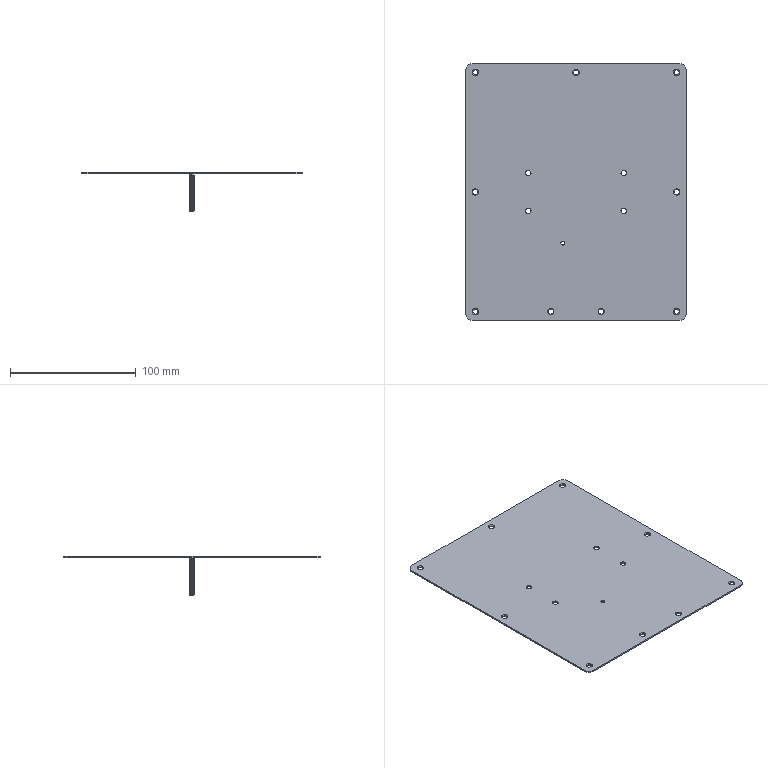Part | SolidWorks | features Chamfer 2, Extrusion 1, Helix 1, ICE 1, SweepCut 1 | 1 solid | 122 faces | box 175 x 204 x 31.2 mm | volume 42842 mm3 | cylinder 91 | cone 20 | plane 8 | spline 3 | commonest cylinder face diameters 3.8 x59 4 x18 4.5 x8 10 x4 3 x2